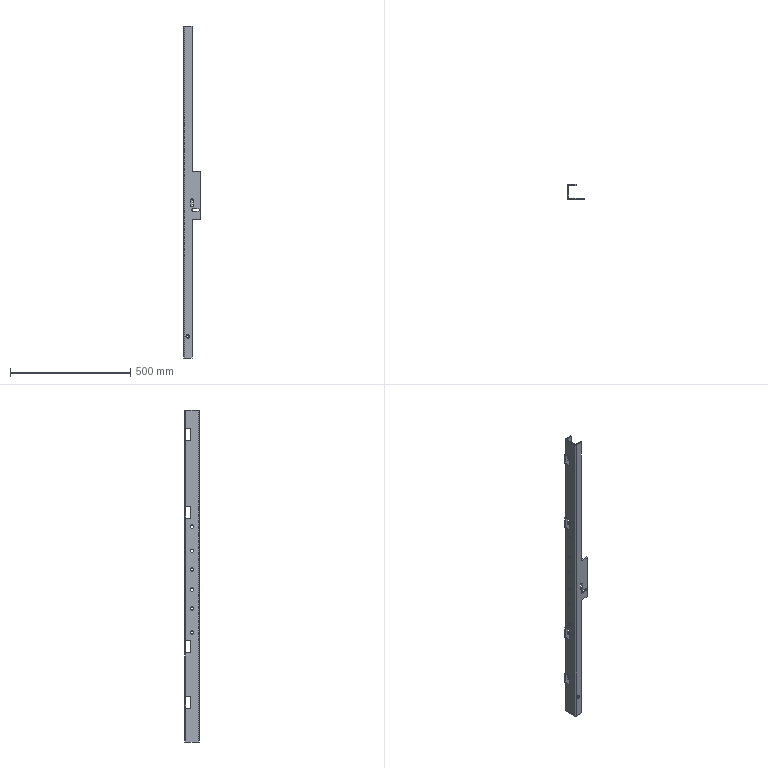Part | SolidWorks | features ICE 10, SMBaseFlange 5, Cut 1, FlatPattern 1, SheetMetal 1 | 1 solid | 129 faces | box 70 x 62 x 1380 mm | volume 672771 mm3 | plane 84 | cylinder 45 | commonest cylinder face diameters 10 x12 14.5 x12 0.4 x6 8.4 x6 12 x5 11 x2